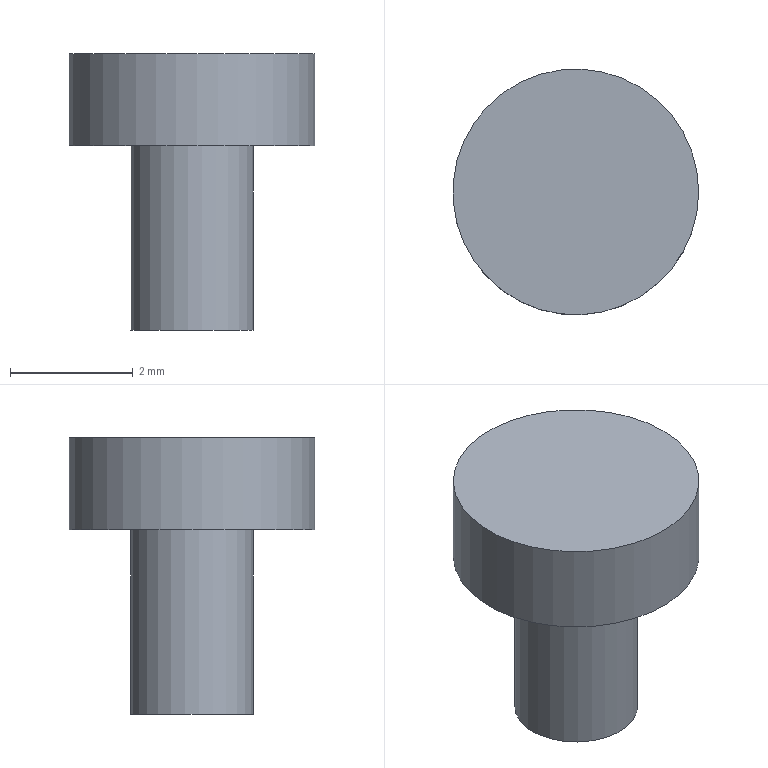Part | NX | features DATUM_CSYS 3, EXTRUDE 2, SKETCH 2 | 1 solid | 5 faces | box 4 x 4 x 4.5 mm | volume 28.274 mm3 | plane 3 | cylinder 2 | commonest cylinder face diameters 2 x1 4 x1
STEP:
#1=CARTESIAN_POINT('',(1.,0.,3.));
#2=VERTEX_POINT('',#1);
#3=CARTESIAN_POINT('',(0.,0.,3.));
#4=DIRECTION('',(0.,0.,1.));
#5=DIRECTION('',(1.,0.,0.));
#6=AXIS2_PLACEMENT_3D('',#3,#4,#5);
#7=CIRCLE('',#6,1.);
#8=EDGE_CURVE('',#2,#2,#7,.T.);
#9=ORIENTED_EDGE('',*,*,#8,.F.);
#10=EDGE_LOOP('',(#9));
#11=FACE_BOUND('',#10,.T.);
#12=CARTESIAN_POINT('',(1.,0.,0.));
#13=VERTEX_POINT('',#12);
#14=CARTESIAN_POINT('',(0.,0.,0.));
#15=DIRECTION('',(0.,0.,1.));
#16=DIRECTION('',(1.,0.,0.));
#17=AXIS2_PLACEMENT_3D('',#14,#15,#16);
#18=CIRCLE('',#17,1.);
#19=EDGE_CURVE('',#13,#13,#18,.T.);
#20=ORIENTED_EDGE('',*,*,#19,.T.);
#21=EDGE_LOOP('',(#20));
#22=FACE_BOUND('',#21,.T.);
#23=CARTESIAN_POINT('',(0.,0.,3.));
#24=DIRECTION('',(0.,0.,-1.));
#25=DIRECTION('',(-1.,0.,0.));
#26=AXIS2_PLACEMENT_3D('',#23,#24,#25);
#27=CYLINDRICAL_SURFACE('',#26,1.);
#28=ADVANCED_FACE('',(#11,#22),#27,.T.);
#29=ORIENTED_EDGE('',*,*,#19,.F.);
#30=EDGE_LOOP('',(#29));
#31=FACE_BOUND('',#30,.T.);
#32=CARTESIAN_POINT('',(0.,0.,0.));
#33=DIRECTION('',(0.,0.,1.));
#34=DIRECTION('',(1.,0.,0.));
#35=AXIS2_PLACEMENT_3D('',#32,#33,#34);
#36=PLANE('',#35);
#37=ADVANCED_FACE('',(#31),#36,.F.);
#38=CARTESIAN_POINT('',(2.,0.,4.5));
#39=VERTEX_POINT('',#38);
#40=CARTESIAN_POINT('',(0.,0.,4.5));
#41=DIRECTION('',(0.,0.,1.));
#42=DIRECTION('',(1.,0.,0.));
#43=AXIS2_PLACEMENT_3D('',#40,#41,#42);
#44=CIRCLE('',#43,2.);
#45=EDGE_CURVE('',#39,#39,#44,.T.);
#46=ORIENTED_EDGE('',*,*,#45,.F.);
#47=EDGE_LOOP('',(#46));
#48=FACE_BOUND('',#47,.T.);
#49=CARTESIAN_POINT('',(2.,0.,3.));
#50=VERTEX_POINT('',#49);
#51=CARTESIAN_POINT('',(0.,0.,3.));
#52=DIRECTION('',(0.,0.,1.));
#53=DIRECTION('',(1.,0.,0.));
#54=AXIS2_PLACEMENT_3D('',#51,#52,#53);
#55=CIRCLE('',#54,2.);
#56=EDGE_CURVE('',#50,#50,#55,.T.);
#57=ORIENTED_EDGE('',*,*,#56,.T.);
#58=EDGE_LOOP('',(#57));
#59=FACE_BOUND('',#58,.T.);
#60=CARTESIAN_POINT('',(0.,0.,4.5));
#61=DIRECTION('',(0.,0.,-1.));
#62=DIRECTION('',(-1.,0.,0.));
#63=AXIS2_PLACEMENT_3D('',#60,#61,#62);
#64=CYLINDRICAL_SURFACE('',#63,2.);
#65=ADVANCED_FACE('',(#48,#59),#64,.T.);
#66=ORIENTED_EDGE('',*,*,#45,.T.);
#67=EDGE_LOOP('',(#66));
#68=FACE_BOUND('',#67,.T.);
#69=CARTESIAN_POINT('',(0.,0.,4.5));
#70=DIRECTION('',(0.,0.,1.));
#71=DIRECTION('',(1.,0.,0.));
#72=AXIS2_PLACEMENT_3D('',#69,#70,#71);
#73=PLANE('',#72);
#74=ADVANCED_FACE('',(#68),#73,.T.);
#75=ORIENTED_EDGE('',*,*,#8,.T.);
#76=EDGE_LOOP('',(#75));
#77=FACE_BOUND('',#76,.T.);
#78=ORIENTED_EDGE('',*,*,#56,.F.);
#79=EDGE_LOOP('',(#78));
#80=FACE_BOUND('',#79,.T.);
#81=CARTESIAN_POINT('',(0.,0.,3.));
#82=DIRECTION('',(0.,0.,1.));
#83=DIRECTION('',(1.,0.,0.));
#84=AXIS2_PLACEMENT_3D('',#81,#82,#83);
#85=PLANE('',#84);
#86=ADVANCED_FACE('',(#77,#80),#85,.F.);
#87=CLOSED_SHELL('',(#28,#37,#65,#74,#86));
#88=MANIFOLD_SOLID_BREP('',#87);
#89=(LENGTH_UNIT()NAMED_UNIT(*)SI_UNIT(.MILLI.,.METRE.));
#90=UNCERTAINTY_MEASURE_WITH_UNIT(LENGTH_MEASURE(0.00001),#89,'','');
#91=(NAMED_UNIT(*)PLANE_ANGLE_UNIT()SI_UNIT($,.RADIAN.));
#92=(NAMED_UNIT(*)SI_UNIT($,.STERADIAN.)SOLID_ANGLE_UNIT());
#93=(GEOMETRIC_REPRESENTATION_CONTEXT(3)GLOBAL_UNCERTAINTY_ASSIGNED_CONTEXT((#90))GLOBAL_UNIT_ASSIGNED_CONTEXT((#89,#91,#92))REPRESENTATION_CONTEXT('',''));
#94=ADVANCED_BREP_SHAPE_REPRESENTATION('',(#88),#93);